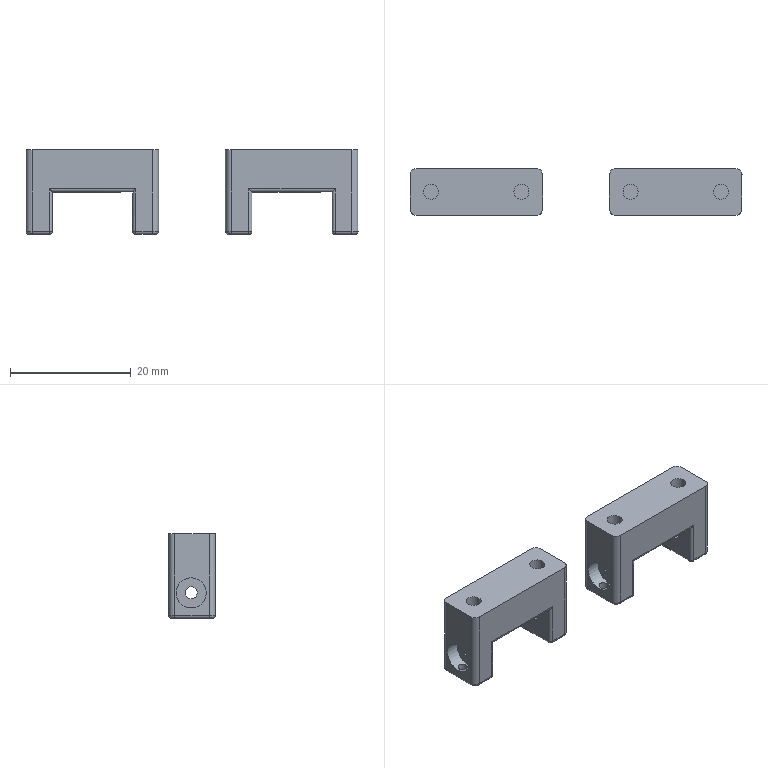CAM job | NX | 3-axis milling | part box 54.928 x 7.717 x 14 mm | stock box 59.928 x 10.717 x 20 mm
Tools:
number,name,description,diameter,corner_radius,flute_length,length,flutes
6,D6,平底铣刀-粗,6.0,0.0,25.0,75.0,2
9,D10,平底铣刀-粗,10.0,0.0,35.0,75.0,2
7,D6-J,平底铣刀-精,6.0,0.0,25.0,75.0,2
17,D4R0.5,圆鼻刀-粗,4.0,0.5,50.0,75.0,2
1,D80R0.8飞刀,圆鼻刀-粗,80.0,0.8,50.0,75.0,2
Operations:
program,operation,operation_type,tool,method,geometry_group,spindle_rpm,surface_speed,feed_per_tooth,feed_cut,feed_plunge,cut_length_mm,path_length_mm,cut_time_min,machine_time_min
A,顶面,FaceMilling,D80R0.8飞刀,侧刃精光-切深K-步距G,W-A,4000.0,1005.31,0.125,1000.0,100.0,148.928,184.928,0.1489,0.1525
A,外形粗_2,VolumeBased25DMillingOperation,D10,METHOD,W-A,8000.0,251.327,0.3125,5000.0,80.0,3587.778,3727.278,0.7176,0.7315
A,底壁粗_1,VolumeBased25DMillingOperation,D6,METHOD,W-A,6000.0,75.398,0.1,1200.0,100.0,2696.413,3301.325,2.247,2.308
A,等高螺旋爬面_COPY,ZLevelMilling,D4R0.5,等高爬面-切深K-步距G,W-A,7000.0,87.965,0.2857,4000.0,100.0,2529.612,2741.951,0.6324,0.6536
A,底精_1,VolumeBased25DMillingOperation,D6-J,METHOD,W-A,6000.0,113.0,0.2083,1200.0,100.0,103.637,241.944,0.0864,0.1002
A,等高精光往复爬面_COPY,ZLevelMilling,D6-J,等高爬面-切深K-步距G,W-A,7000.0,131.947,0.2857,4000.0,100.0,2374.037,2608.404,0.5935,0.6169
A,等高精光-中_COPY,ZLevelMilling,D6-J,侧刃精光-切深K-步距G,W-A,8000.0,150.792,0.0625,1000.0,100.0,402.772,805.467,0.4028,0.443